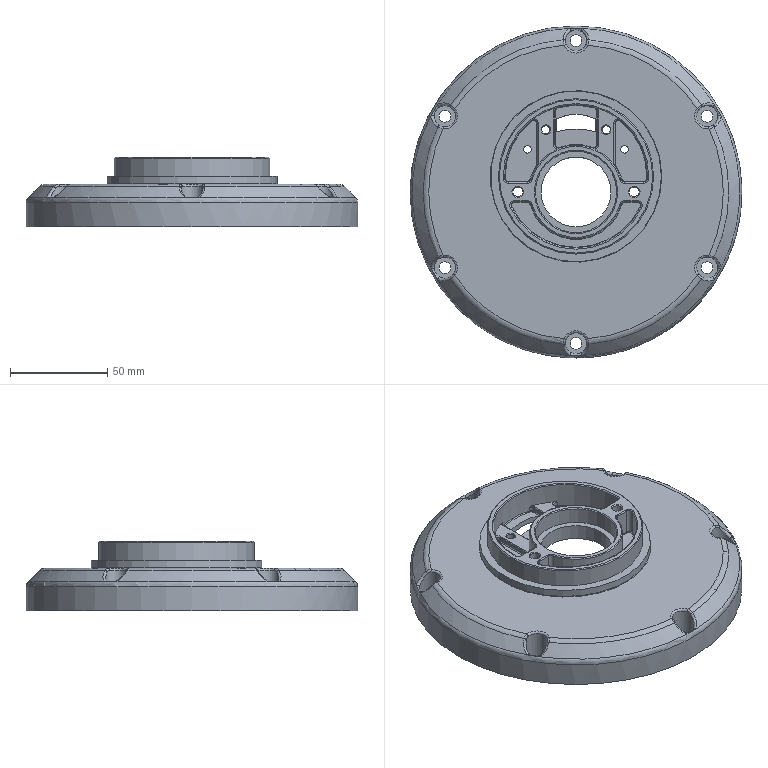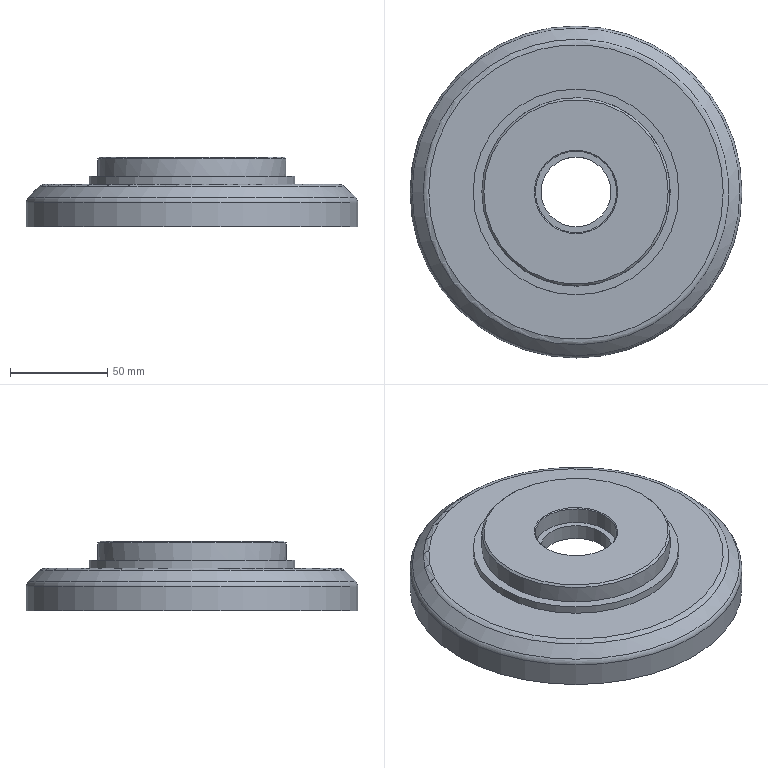CAM job | NX | 3-axis milling, drilling | part box 171 x 171 x 36 mm | stock box 171 x 171 x 36 mm
Tools:
number,name,description,diameter,corner_radius,flute_length,length,flutes
1,D12-L45,,12.0,0.0,40.0,45.0,2
6,D6-L25,,6.0,0.0,20.0,25.0,2
8,D4-L24,,4.0,0.0,12.0,24.0,2
15,C8-L35,,8.0,0.0,25.0,35.0,2
16,DK-3.5-L30,,3.5,0.0,25.0,30.0,2
17,DK-4.2-L35,,4.2,0.0,30.0,35.0,2
18,DK-5.5-L40,,5.5,0.0,35.0,40.0,2
19,DK-5.0-L40,,5.0,0.0,35.0,40.0,2
10,D2R1-L15,,2.0,1.0,10.0,15.0,2
2,D12J-L45,,12.0,0.0,40.0,45.0,2
9,D4J-L24,,4.0,0.0,20.0,24.0,2
11,D10R0.2-L30,,10.0,0.2,20.0,30.0,2
14,DJ-8-L30,,8.0,0.0,20.0,30.0,2
20,M5X0.8-L30,,4.2,0.0,20.0,30.0,4
21,M6X1-L30,,5.0,0.0,20.0,30.0,4
0,R2,,3.8,1.9,50.0,75.0,2
Operations:
program,operation,operation_type,tool,method,geometry_group,spindle_rpm,surface_speed,feed_per_tooth,feed_cut,feed_plunge,cut_length_mm,path_length_mm,cut_time_min,machine_time_min
A-01,动态加工0.5,CavityMilling,D12-L45,METHOD,W-11,4000.0,100.0,0.1178,2500.0,100.0,31721.582,32681.413,10.416,10.512
A-01,3D开粗,CavityMilling,D6-L25,METHOD,W-11,4500.0,100.0,0.1178,2500.0,100.0,18677.385,22867.161,7.471,7.799
A-01,3D开粗_COPY,CavityMilling,D6-L25,METHOD,W-11,4500.0,100.0,0.1178,2500.0,100.0,15575.488,17994.621,6.23,6.418
A-01,3D开粗_COPY_COPY,CavityMilling,D4-L24,METHOD,W-11,5000.0,100.0,0.1178,2500.0,100.0,12201.243,15332.187,4.88,5.135
A-01,点孔-A,Operation,C8-L35,NONE,W-11,1500.0,75.0,0.0283,120.0,0.0,21.0,546.128,0.175,0.2275
A-01,点孔-A_COPY_1,Operation,C8-L35,NONE,W-11,1500.0,75.0,0.0283,120.0,0.0,7.0,109.064,0.0583,0.0685
A-01,点孔-A_COPY_1_COPY_1,Operation,C8-L35,NONE,W-11,1500.0,75.0,0.0283,120.0,0.0,14.0,225.732,0.1167,0.1378
A-01,点孔-A_COPY_1_COPY_1_COPY,Operation,DK-3.5-L30,NONE,W-11,1200.0,75.0,0.0283,70.0,0.0,14.103,148.246,0.2015,0.2149
A-01,点孔-A_COPY_1_COPY,Operation,DK-4.2-L35,NONE,W-11,1200.0,75.0,0.0283,50.0,0.0,20.524,136.112,0.4105,0.422
A-01,点孔-A_COPY,Operation,DK-5.5-L40,NONE,W-11,900.0,75.0,0.0283,70.0,0.0,51.914,607.957,0.7416,0.7972
A-01,点孔-A_COPY_COPY,Operation,DK-5.0-L40,NONE,W-11,900.0,75.0,0.0283,70.0,0.0,43.004,188.042,0.6143,0.6289
A-01,点孔-A_COPY_1_COPY_1_COPY_1,Operation,C8-L35,NONE,W-11,2500.0,75.0,0.0283,150.0,0.0,9.6,121.233,0.064,0.0752
A-01,点孔-A_COPY_1_COPY_1_COPY_1_COPY,Operation,C8-L35,NONE,W-11,2500.0,75.0,0.0283,150.0,0.0,8.6,112.264,0.0573,0.0677
A-01,点孔-A_COPY_1_COPY_1_COPY_1_COPY_COPY,Operation,C8-L35,NONE,W-11,2500.0,75.0,0.0283,150.0,0.0,8.0,136.04,0.0533,0.0661
A-01,点孔-A_COPY_2,Operation,C8-L35,NONE,W-11,2500.0,75.0,0.0283,150.0,0.0,30.0,564.128,0.2,0.2534
A-01,铣孔-0.12,CylinderMilling,D4-L24,METHOD,W-11,3500.0,100.0,0.1178,1200.0,100.0,480.155,1515.155,0.4001,0.5036
A-01,区域铣削,SurfaceContour,D2R1-L15,METHOD,W-11,4500.0,100.0,0.1178,1500.0,100.0,10364.886,10989.437,6.91,6.972
A-01,引导曲线,SurfaceContour,D2R1-L15,METHOD,W-11,5000.0,100.0,0.1178,2000.0,100.0,5422.607,5462.111,2.711,2.715
A-01,引导曲线_COPY,SurfaceContour,D2R1-L15,METHOD,W-11,5000.0,100.0,0.1178,2000.0,100.0,6696.232,6735.703,3.348,3.352
A-01,底壁铣开粗,VolumeBased25DMillingOperation,D12J-L45,METHOD,W-11,4000.0,100.0,0.1178,800.0,100.0,311.741,370.741,0.3897,0.3956
A-01,D02,VolumeBased25DMillingOperation,D12J-L45,METHOD,W-11,4000.0,100.0,0.1178,800.0,100.0,310.79,369.79,0.3885,0.3944
A-01,底壁铣开粗_COPY_COPY_1,VolumeBased25DMillingOperation,D4J-L24,METHOD,W-11,4500.0,100.0,0.1178,700.0,100.0,259.001,404.667,0.37,0.3846
A-01,底壁铣开粗_COPY_COPY_1_COPY,VolumeBased25DMillingOperation,D4J-L24,METHOD,W-11,4000.0,100.0,0.1178,600.0,100.0,218.509,550.431,0.3642,0.3939
A-01,D08,CylinderMilling,D4J-L24,METHOD,W-11,2500.0,100.0,0.1178,200.0,100.0,224.483,1259.483,1.122,1.226
A-01,铣孔-0.12_COPY,CylinderMilling,D4J-L24,METHOD,W-11,3500.0,100.0,0.1178,800.0,100.0,2512.377,3421.377,3.14,3.231
A-01,底壁铣开粗_COPY_1,VolumeBased25DMillingOperation,D4J-L24,METHOD,W-11,4000.0,100.0,0.1178,600.0,100.0,147.724,215.124,0.2462,0.2529
A-01,底壁铣开粗_COPY_1_COPY,VolumeBased25DMillingOperation,D4J-L24,METHOD,W-11,4000.0,100.0,0.1178,600.0,100.0,325.992,491.638,0.5433,0.5599
A-01,底壁铣开粗_COPY_1_COPY_COPY,VolumeBased25DMillingOperation,D4J-L24,METHOD,W-11,4000.0,100.0,0.1178,600.0,100.0,147.679,337.661,0.2461,0.2651
A-01,等高爬倒角,ZLevelMilling,D4J-L24,METHOD,W-11,4500.0,100.0,0.1178,700.0,100.0,1456.183,1939.804,2.08,2.129
A-01,等高爬倒角_COPY,ZLevelMilling,D4J-L24,METHOD,W-11,4500.0,100.0,0.1178,1500.0,100.0,816.264,1173.995,0.5442,0.58
A-01,底壁铣开粗_COPY,VolumeBased25DMillingOperation,D10R0.2-L30,METHOD,W-11,4000.0,100.0,0.1178,750.0,100.0,1302.457,1369.358,1.737,1.743
A-01,底壁铣开粗_COPY_COPY,VolumeBased25DMillingOperation,D10R0.2-L30,METHOD,W-11,4000.0,100.0,0.1178,750.0,100.0,322.614,389.514,0.4302,0.4368
A-01,轮廓倒角-01,PlanarMilling,DJ-8-L30,NONE,W-11,3000.0,0.0,0.0,800.0,100.0,264.394,308.394,0.3305,0.3349
A-01,轮廓倒角-01_COPY,PlanarMilling,DJ-8-L30,NONE,W-11,3000.0,0.0,0.0,800.0,100.0,292.668,356.668,0.3658,0.3722
A-01,点孔-A_COPY_1_COPY_COPY,Operation,M5X0.8-L30,NONE,W-11,200.0,75.0,0.0283,0.8,0.0,14.0,123.064,17.5,17.511
A-01,点孔-A_COPY_1_COPY_COPY_COPY,Operation,M6X1-L30,NONE,W-11,200.0,75.0,0.0283,1.0,0.0,14.0,130.033,14.0,14.012
A-03,底壁铣开粗_COPY_1_COPY_COPY_1,VolumeBased25DMillingOperation,D4J-L24,METHOD,11,4000.0,50.0,0.075,600.0,100.0,387.296,738.815,0.6455,0.6806
A-03,底壁铣开粗_COPY_COPY_2,VolumeBased25DMillingOperation,D10R0.2-L30,METHOD,W-11,4000.0,100.0,0.1178,750.0,100.0,1302.457,1369.358,1.737,1.743
A-03,底壁铣开粗_COPY_COPY_COPY,VolumeBased25DMillingOperation,D10R0.2-L30,METHOD,W-11,4000.0,100.0,0.1178,750.0,100.0,322.614,389.514,0.4302,0.4368
一般加工工序,动态加工0.5_1,CavityMilling,D12-L45,METHOD,W-22,3500.0,131.0,0.2143,1500.0,100.0,61174.331,64482.243,29.374,29.705
一般加工工序,动态加工0.5_1_COPY,CavityMilling,D4-L24,METHOD,W-22,3000.0,37.0,0.1667,1000.0,100.0,11783.874,23960.695,10.494,11.712
一般加工工序,PLANAR_MILL,PlanarMilling,D4J-L24,METHOD,W-22,3000.0,37.0,0.1,600.0,100.0,3150.077,3206.42,5.25,5.256
一般加工工序,PLANAR_MILL_COPY,PlanarMilling,D4J-L24,METHOD,W-22,3000.0,37.0,0.1,600.0,100.0,633.732,690.075,1.056,1.062
一般加工工序,AREA_MILL,SurfaceContour,R2,METHOD,W-22,3500.0,43.0,0.3571,2500.0,100.0,145232.193,146976.492,58.093,58.267